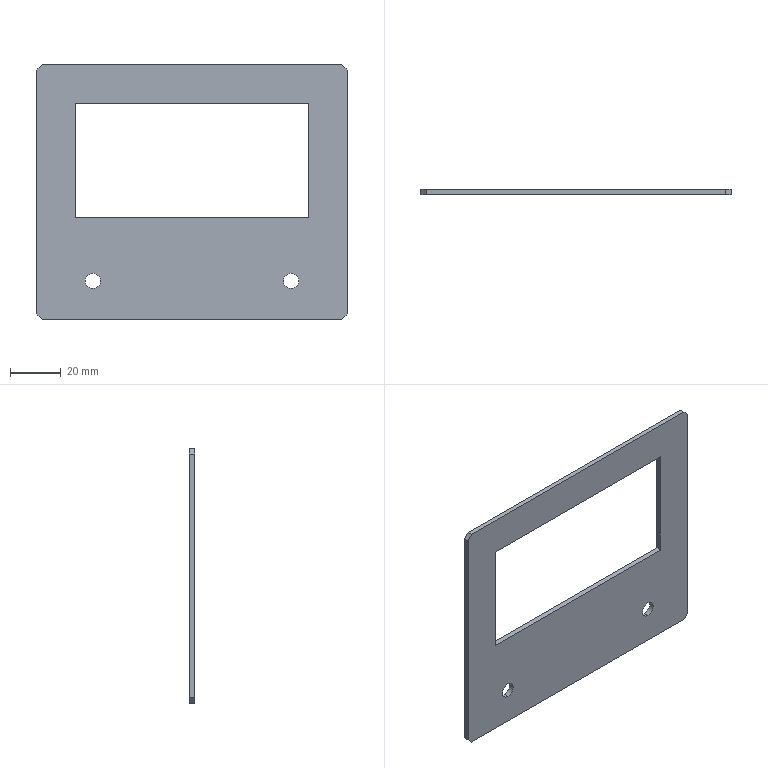Part | STEP file | 227H0563998 BKT_Default | 1 solid | 18 faces | box 122 x 2 x 100 mm | volume 15991 mm3 | plane 14 | cylinder 4 | commonest cylinder face diameters 6 x4
STEP:
#1=CARTESIAN_POINT('',(0.,0.,0.));
#2=DIRECTION('',(0.,0.,1.));
#3=DIRECTION('',(1.,0.,0.));
#4=AXIS2_PLACEMENT_3D('',#1,#2,#3);
#5=CARTESIAN_POINT('',(39.,-2.,-32.));
#6=VERTEX_POINT('',#5);
#7=CARTESIAN_POINT('',(39.,0.,-32.));
#8=VERTEX_POINT('',#7);
#9=CARTESIAN_POINT('',(39.,0.,-32.));
#10=DIRECTION('',(0.,1.,0.));
#11=VECTOR('',#10,1.);
#12=LINE('',#9,#11);
#13=CARTESIAN_POINT('',(39.,0.,-35.));
#14=DIRECTION('',(0.,1.,0.));
#15=DIRECTION('',(0.,0.,1.));
#16=AXIS2_PLACEMENT_3D('',#13,#14,#15);
#17=CYLINDRICAL_SURFACE('',#16,3.);
#18=CARTESIAN_POINT('',(6.283,0.));
#19=DIRECTION('',(0.,1.));
#20=VECTOR('',#19,1.);
#21=LINE('',#18,#20);
#22=(GEOMETRIC_REPRESENTATION_CONTEXT(2)PARAMETRIC_REPRESENTATION_CONTEXT()REPRESENTATION_CONTEXT('',''));
#23=DEFINITIONAL_REPRESENTATION('',(#21),#22);
#24=PCURVE('',#17,#23);
#25=CARTESIAN_POINT('',(39.,0.,-35.));
#26=DIRECTION('',(0.,1.,0.));
#27=DIRECTION('',(0.,0.,1.));
#28=AXIS2_PLACEMENT_3D('',#25,#26,#27);
#29=CYLINDRICAL_SURFACE('',#28,3.);
#30=CARTESIAN_POINT('',(0.,0.));
#31=DIRECTION('',(0.,1.));
#32=VECTOR('',#31,1.);
#33=LINE('',#30,#32);
#34=(GEOMETRIC_REPRESENTATION_CONTEXT(2)PARAMETRIC_REPRESENTATION_CONTEXT()REPRESENTATION_CONTEXT('',''));
#35=DEFINITIONAL_REPRESENTATION('',(#33),#34);
#36=PCURVE('',#29,#35);
#37=SURFACE_CURVE('',#12,(#24,#36),.PCURVE_S1.);
#38=EDGE_CURVE('',#6,#8,#37,.T.);
#39=ORIENTED_EDGE('',*,*,#38,.T.);
#40=CARTESIAN_POINT('',(39.,0.,-38.));
#41=VERTEX_POINT('',#40);
#42=CARTESIAN_POINT('',(39.,0.,-35.));
#43=DIRECTION('',(0.,1.,0.));
#44=DIRECTION('',(0.,0.,1.));
#45=AXIS2_PLACEMENT_3D('',#42,#43,#44);
#46=CIRCLE('',#45,3.);
#47=CARTESIAN_POINT('',(0.,0.));
#48=DIRECTION('',(1.,0.));
#49=VECTOR('',#48,1.);
#50=LINE('',#47,#49);
#51=(GEOMETRIC_REPRESENTATION_CONTEXT(2)PARAMETRIC_REPRESENTATION_CONTEXT()REPRESENTATION_CONTEXT('',''));
#52=DEFINITIONAL_REPRESENTATION('',(#50),#51);
#53=PCURVE('',#17,#52);
#54=CARTESIAN_POINT('',(0.,0.,0.));
#55=DIRECTION('',(0.,1.,0.));
#56=DIRECTION('',(0.,0.,1.));
#57=AXIS2_PLACEMENT_3D('',#54,#55,#56);
#58=PLANE('',#57);
#59=CARTESIAN_POINT('',(-35.,39.));
#60=DIRECTION('',(1.,0.));
#61=AXIS2_PLACEMENT_2D('',#59,#60);
#62=CIRCLE('',#61,3.);
#63=(GEOMETRIC_REPRESENTATION_CONTEXT(2)PARAMETRIC_REPRESENTATION_CONTEXT()REPRESENTATION_CONTEXT('',''));
#64=DEFINITIONAL_REPRESENTATION('',(#62),#63);
#65=PCURVE('',#58,#64);
#66=SURFACE_CURVE('',#46,(#53,#65),.PCURVE_S1.);
#67=EDGE_CURVE('',#41,#8,#66,.T.);
#68=ORIENTED_EDGE('',*,*,#67,.F.);
#69=CARTESIAN_POINT('',(39.,-2.,-38.));
#70=VERTEX_POINT('',#69);
#71=CARTESIAN_POINT('',(39.,0.,-38.));
#72=DIRECTION('',(0.,1.,0.));
#73=VECTOR('',#72,1.);
#74=LINE('',#71,#73);
#75=CARTESIAN_POINT('',(3.142,0.));
#76=DIRECTION('',(0.,1.));
#77=VECTOR('',#76,1.);
#78=LINE('',#75,#77);
#79=(GEOMETRIC_REPRESENTATION_CONTEXT(2)PARAMETRIC_REPRESENTATION_CONTEXT()REPRESENTATION_CONTEXT('',''));
#80=DEFINITIONAL_REPRESENTATION('',(#78),#79);
#81=PCURVE('',#17,#80);
#82=CARTESIAN_POINT('',(3.142,0.));
#83=DIRECTION('',(0.,1.));
#84=VECTOR('',#83,1.);
#85=LINE('',#82,#84);
#86=(GEOMETRIC_REPRESENTATION_CONTEXT(2)PARAMETRIC_REPRESENTATION_CONTEXT()REPRESENTATION_CONTEXT('',''));
#87=DEFINITIONAL_REPRESENTATION('',(#85),#86);
#88=PCURVE('',#29,#87);
#89=SURFACE_CURVE('',#74,(#81,#88),.PCURVE_S1.);
#90=EDGE_CURVE('',#70,#41,#89,.T.);
#91=ORIENTED_EDGE('',*,*,#90,.F.);
#92=CARTESIAN_POINT('',(39.,-2.,-35.));
#93=DIRECTION('',(0.,1.,0.));
#94=DIRECTION('',(0.,0.,1.));
#95=AXIS2_PLACEMENT_3D('',#92,#93,#94);
#96=CIRCLE('',#95,3.);
#97=CARTESIAN_POINT('',(0.,-2.));
#98=DIRECTION('',(1.,0.));
#99=VECTOR('',#98,1.);
#100=LINE('',#97,#99);
#101=(GEOMETRIC_REPRESENTATION_CONTEXT(2)PARAMETRIC_REPRESENTATION_CONTEXT()REPRESENTATION_CONTEXT('',''));
#102=DEFINITIONAL_REPRESENTATION('',(#100),#101);
#103=PCURVE('',#17,#102);
#104=CARTESIAN_POINT('',(0.,-2.,0.));
#105=DIRECTION('',(0.,1.,0.));
#106=DIRECTION('',(0.,0.,1.));
#107=AXIS2_PLACEMENT_3D('',#104,#105,#106);
#108=PLANE('',#107);
#109=CARTESIAN_POINT('',(-35.,39.));
#110=DIRECTION('',(1.,0.));
#111=AXIS2_PLACEMENT_2D('',#109,#110);
#112=CIRCLE('',#111,3.);
#113=(GEOMETRIC_REPRESENTATION_CONTEXT(2)PARAMETRIC_REPRESENTATION_CONTEXT()REPRESENTATION_CONTEXT('',''));
#114=DEFINITIONAL_REPRESENTATION('',(#112),#113);
#115=PCURVE('',#108,#114);
#116=SURFACE_CURVE('',#96,(#103,#115),.PCURVE_S1.);
#117=EDGE_CURVE('',#70,#6,#116,.T.);
#118=ORIENTED_EDGE('',*,*,#117,.T.);
#119=EDGE_LOOP('',(#39,#68,#91,#118));
#120=FACE_BOUND('',#119,.F.);
#121=ADVANCED_FACE('',(#120),#17,.F.);
#122=CARTESIAN_POINT('',(-39.,-2.,-32.));
#123=VERTEX_POINT('',#122);
#124=CARTESIAN_POINT('',(-39.,0.,-32.));
#125=VERTEX_POINT('',#124);
#126=CARTESIAN_POINT('',(-39.,0.,-32.));
#127=DIRECTION('',(0.,1.,0.));
#128=VECTOR('',#127,1.);
#129=LINE('',#126,#128);
#130=CARTESIAN_POINT('',(-39.,0.,-35.));
#131=DIRECTION('',(0.,1.,0.));
#132=DIRECTION('',(0.,0.,1.));
#133=AXIS2_PLACEMENT_3D('',#130,#131,#132);
#134=CYLINDRICAL_SURFACE('',#133,3.);
#135=CARTESIAN_POINT('',(6.283,0.));
#136=DIRECTION('',(0.,1.));
#137=VECTOR('',#136,1.);
#138=LINE('',#135,#137);
#139=(GEOMETRIC_REPRESENTATION_CONTEXT(2)PARAMETRIC_REPRESENTATION_CONTEXT()REPRESENTATION_CONTEXT('',''));
#140=DEFINITIONAL_REPRESENTATION('',(#138),#139);
#141=PCURVE('',#134,#140);
#142=CARTESIAN_POINT('',(-39.,0.,-35.));
#143=DIRECTION('',(0.,1.,0.));
#144=DIRECTION('',(0.,0.,1.));
#145=AXIS2_PLACEMENT_3D('',#142,#143,#144);
#146=CYLINDRICAL_SURFACE('',#145,3.);
#147=CARTESIAN_POINT('',(0.,0.));
#148=DIRECTION('',(0.,1.));
#149=VECTOR('',#148,1.);
#150=LINE('',#147,#149);
#151=(GEOMETRIC_REPRESENTATION_CONTEXT(2)PARAMETRIC_REPRESENTATION_CONTEXT()REPRESENTATION_CONTEXT('',''));
#152=DEFINITIONAL_REPRESENTATION('',(#150),#151);
#153=PCURVE('',#146,#152);
#154=SURFACE_CURVE('',#129,(#141,#153),.PCURVE_S1.);
#155=EDGE_CURVE('',#123,#125,#154,.T.);
#156=ORIENTED_EDGE('',*,*,#155,.T.);
#157=CARTESIAN_POINT('',(-39.,0.,-38.));
#158=VERTEX_POINT('',#157);
#159=CARTESIAN_POINT('',(-39.,0.,-35.));
#160=DIRECTION('',(0.,1.,0.));
#161=DIRECTION('',(0.,0.,1.));
#162=AXIS2_PLACEMENT_3D('',#159,#160,#161);
#163=CIRCLE('',#162,3.);
#164=CARTESIAN_POINT('',(0.,0.));
#165=DIRECTION('',(1.,0.));
#166=VECTOR('',#165,1.);
#167=LINE('',#164,#166);
#168=(GEOMETRIC_REPRESENTATION_CONTEXT(2)PARAMETRIC_REPRESENTATION_CONTEXT()REPRESENTATION_CONTEXT('',''));
#169=DEFINITIONAL_REPRESENTATION('',(#167),#168);
#170=PCURVE('',#134,#169);
#171=CARTESIAN_POINT('',(-35.,-39.));
#172=DIRECTION('',(1.,0.));
#173=AXIS2_PLACEMENT_2D('',#171,#172);
#174=CIRCLE('',#173,3.);
#175=(GEOMETRIC_REPRESENTATION_CONTEXT(2)PARAMETRIC_REPRESENTATION_CONTEXT()REPRESENTATION_CONTEXT('',''));
#176=DEFINITIONAL_REPRESENTATION('',(#174),#175);
#177=PCURVE('',#58,#176);
#178=SURFACE_CURVE('',#163,(#170,#177),.PCURVE_S1.);
#179=EDGE_CURVE('',#158,#125,#178,.T.);
#180=ORIENTED_EDGE('',*,*,#179,.F.);
#181=CARTESIAN_POINT('',(-39.,-2.,-38.));
#182=VERTEX_POINT('',#181);
#183=CARTESIAN_POINT('',(-39.,0.,-38.));
#184=DIRECTION('',(0.,1.,0.));
#185=VECTOR('',#184,1.);
#186=LINE('',#183,#185);
#187=CARTESIAN_POINT('',(3.142,0.));
#188=DIRECTION('',(0.,1.));
#189=VECTOR('',#188,1.);
#190=LINE('',#187,#189);
#191=(GEOMETRIC_REPRESENTATION_CONTEXT(2)PARAMETRIC_REPRESENTATION_CONTEXT()REPRESENTATION_CONTEXT('',''));
#192=DEFINITIONAL_REPRESENTATION('',(#190),#191);
#193=PCURVE('',#134,#192);
#194=CARTESIAN_POINT('',(3.142,0.));
#195=DIRECTION('',(0.,1.));
#196=VECTOR('',#195,1.);
#197=LINE('',#194,#196);
#198=(GEOMETRIC_REPRESENTATION_CONTEXT(2)PARAMETRIC_REPRESENTATION_CONTEXT()REPRESENTATION_CONTEXT('',''));
#199=DEFINITIONAL_REPRESENTATION('',(#197),#198);
#200=PCURVE('',#146,#199);
#201=SURFACE_CURVE('',#186,(#193,#200),.PCURVE_S1.);
#202=EDGE_CURVE('',#182,#158,#201,.T.);
#203=ORIENTED_EDGE('',*,*,#202,.F.);
#204=CARTESIAN_POINT('',(-39.,-2.,-35.));
#205=DIRECTION('',(0.,1.,0.));
#206=DIRECTION('',(0.,0.,1.));
#207=AXIS2_PLACEMENT_3D('',#204,#205,#206);
#208=CIRCLE('',#207,3.);
#209=CARTESIAN_POINT('',(0.,-2.));
#210=DIRECTION('',(1.,0.));
#211=VECTOR('',#210,1.);
#212=LINE('',#209,#211);
#213=(GEOMETRIC_REPRESENTATION_CONTEXT(2)PARAMETRIC_REPRESENTATION_CONTEXT()REPRESENTATION_CONTEXT('',''));
#214=DEFINITIONAL_REPRESENTATION('',(#212),#213);
#215=PCURVE('',#134,#214);
#216=CARTESIAN_POINT('',(-35.,-39.));
#217=DIRECTION('',(1.,0.));
#218=AXIS2_PLACEMENT_2D('',#216,#217);
#219=CIRCLE('',#218,3.);
#220=(GEOMETRIC_REPRESENTATION_CONTEXT(2)PARAMETRIC_REPRESENTATION_CONTEXT()REPRESENTATION_CONTEXT('',''));
#221=DEFINITIONAL_REPRESENTATION('',(#219),#220);
#222=PCURVE('',#108,#221);
#223=SURFACE_CURVE('',#208,(#215,#222),.PCURVE_S1.);
#224=EDGE_CURVE('',#182,#123,#223,.T.);
#225=ORIENTED_EDGE('',*,*,#224,.T.);
#226=EDGE_LOOP('',(#156,#180,#203,#225));
#227=FACE_BOUND('',#226,.F.);
#228=ADVANCED_FACE('',(#227),#134,.F.);
#229=CARTESIAN_POINT('',(-61.,0.,-48.));
#230=VERTEX_POINT('',#229);
#231=CARTESIAN_POINT('',(-61.,0.,48.));
#232=VERTEX_POINT('',#231);
#233=CARTESIAN_POINT('',(-61.,0.,50.));
#234=DIRECTION('',(0.,0.,1.));
#235=VECTOR('',#234,1.);
#236=LINE('',#233,#235);
#237=CARTESIAN_POINT('',(-61.,-2.,50.));
#238=DIRECTION('',(-1.,0.,0.));
#239=DIRECTION('',(0.,0.,1.));
#240=AXIS2_PLACEMENT_3D('',#237,#238,#239);
#241=PLANE('',#240);
#242=CARTESIAN_POINT('',(0.,2.));
#243=DIRECTION('',(1.,0.));
#244=VECTOR('',#243,1.);
#245=LINE('',#242,#244);
#246=(GEOMETRIC_REPRESENTATION_CONTEXT(2)PARAMETRIC_REPRESENTATION_CONTEXT()REPRESENTATION_CONTEXT('',''));
#247=DEFINITIONAL_REPRESENTATION('',(#245),#246);
#248=PCURVE('',#241,#247);
#249=CARTESIAN_POINT('',(50.,-61.));
#250=DIRECTION('',(1.,0.));
#251=VECTOR('',#250,1.);
#252=LINE('',#249,#251);
#253=(GEOMETRIC_REPRESENTATION_CONTEXT(2)PARAMETRIC_REPRESENTATION_CONTEXT()REPRESENTATION_CONTEXT('',''));
#254=DEFINITIONAL_REPRESENTATION('',(#252),#253);
#255=PCURVE('',#58,#254);
#256=SURFACE_CURVE('',#236,(#248,#255),.PCURVE_S1.);
#257=EDGE_CURVE('',#230,#232,#256,.T.);
#258=ORIENTED_EDGE('',*,*,#257,.F.);
#259=CARTESIAN_POINT('',(-61.,-2.,-48.));
#260=VERTEX_POINT('',#259);
#261=CARTESIAN_POINT('',(-61.,-2.,-48.));
#262=DIRECTION('',(0.,-1.,0.));
#263=VECTOR('',#262,1.);
#264=LINE('',#261,#263);
#265=CARTESIAN_POINT('',(-98.,0.));
#266=DIRECTION('',(0.,-1.));
#267=VECTOR('',#266,1.);
#268=LINE('',#265,#267);
#269=(GEOMETRIC_REPRESENTATION_CONTEXT(2)PARAMETRIC_REPRESENTATION_CONTEXT()REPRESENTATION_CONTEXT('',''));
#270=DEFINITIONAL_REPRESENTATION('',(#268),#269);
#271=PCURVE('',#241,#270);
#272=CARTESIAN_POINT('',(-59.,-2.,-50.));
#273=DIRECTION('',(0.7071,0.,0.7071));
#274=DIRECTION('',(0.,1.,0.));
#275=AXIS2_PLACEMENT_3D('',#272,#273,#274);
#276=PLANE('',#275);
#277=CARTESIAN_POINT('',(0.,2.828));
#278=DIRECTION('',(-1.,0.));
#279=VECTOR('',#278,1.);
#280=LINE('',#277,#279);
#281=(GEOMETRIC_REPRESENTATION_CONTEXT(2)PARAMETRIC_REPRESENTATION_CONTEXT()REPRESENTATION_CONTEXT('',''));
#282=DEFINITIONAL_REPRESENTATION('',(#280),#281);
#283=PCURVE('',#276,#282);
#284=SURFACE_CURVE('',#264,(#271,#283),.PCURVE_S1.);
#285=EDGE_CURVE('',#230,#260,#284,.T.);
#286=ORIENTED_EDGE('',*,*,#285,.T.);
#287=CARTESIAN_POINT('',(-61.,-2.,48.));
#288=VERTEX_POINT('',#287);
#289=CARTESIAN_POINT('',(-61.,-2.,50.));
#290=DIRECTION('',(0.,0.,1.));
#291=VECTOR('',#290,1.);
#292=LINE('',#289,#291);
#293=CARTESIAN_POINT('',(0.,0.));
#294=DIRECTION('',(1.,0.));
#295=VECTOR('',#294,1.);
#296=LINE('',#293,#295);
#297=(GEOMETRIC_REPRESENTATION_CONTEXT(2)PARAMETRIC_REPRESENTATION_CONTEXT()REPRESENTATION_CONTEXT('',''));
#298=DEFINITIONAL_REPRESENTATION('',(#296),#297);
#299=PCURVE('',#241,#298);
#300=CARTESIAN_POINT('',(50.,-61.));
#301=DIRECTION('',(1.,0.));
#302=VECTOR('',#301,1.);
#303=LINE('',#300,#302);
#304=(GEOMETRIC_REPRESENTATION_CONTEXT(2)PARAMETRIC_REPRESENTATION_CONTEXT()REPRESENTATION_CONTEXT('',''));
#305=DEFINITIONAL_REPRESENTATION('',(#303),#304);
#306=PCURVE('',#108,#305);
#307=SURFACE_CURVE('',#292,(#299,#306),.PCURVE_S1.);
#308=EDGE_CURVE('',#260,#288,#307,.T.);
#309=ORIENTED_EDGE('',*,*,#308,.T.);
#310=CARTESIAN_POINT('',(-61.,-2.,48.));
#311=DIRECTION('',(0.,1.,0.));
#312=VECTOR('',#311,1.);
#313=LINE('',#310,#312);
#314=CARTESIAN_POINT('',(-2.,0.));
#315=DIRECTION('',(0.,1.));
#316=VECTOR('',#315,1.);
#317=LINE('',#314,#316);
#318=(GEOMETRIC_REPRESENTATION_CONTEXT(2)PARAMETRIC_REPRESENTATION_CONTEXT()REPRESENTATION_CONTEXT('',''));
#319=DEFINITIONAL_REPRESENTATION('',(#317),#318);
#320=PCURVE('',#241,#319);
#321=CARTESIAN_POINT('',(-61.,-2.,48.));
#322=DIRECTION('',(0.7071,0.,-0.7071));
#323=DIRECTION('',(0.,1.,0.));
#324=AXIS2_PLACEMENT_3D('',#321,#322,#323);
#325=PLANE('',#324);
#326=CARTESIAN_POINT('',(0.,0.));
#327=DIRECTION('',(1.,0.));
#328=VECTOR('',#327,1.);
#329=LINE('',#326,#328);
#330=(GEOMETRIC_REPRESENTATION_CONTEXT(2)PARAMETRIC_REPRESENTATION_CONTEXT()REPRESENTATION_CONTEXT('',''));
#331=DEFINITIONAL_REPRESENTATION('',(#329),#330);
#332=PCURVE('',#325,#331);
#333=SURFACE_CURVE('',#313,(#320,#332),.PCURVE_S1.);
#334=EDGE_CURVE('',#288,#232,#333,.T.);
#335=ORIENTED_EDGE('',*,*,#334,.T.);
#336=EDGE_LOOP('',(#258,#286,#309,#335));
#337=FACE_BOUND('',#336,.T.);
#338=ADVANCED_FACE('',(#337),#241,.T.);
#339=CARTESIAN_POINT('',(59.,-2.,-50.));
#340=VERTEX_POINT('',#339);
#341=CARTESIAN_POINT('',(-59.,-2.,-50.));
#342=VERTEX_POINT('',#341);
#343=CARTESIAN_POINT('',(61.,-2.,-50.));
#344=DIRECTION('',(-1.,0.,0.));
#345=VECTOR('',#344,1.);
#346=LINE('',#343,#345);
#347=CARTESIAN_POINT('',(61.,-2.,-50.));
#348=DIRECTION('',(0.,0.,-1.));
#349=DIRECTION('',(-1.,0.,0.));
#350=AXIS2_PLACEMENT_3D('',#347,#348,#349);
#351=PLANE('',#350);
#352=CARTESIAN_POINT('',(0.,0.));
#353=DIRECTION('',(1.,0.));
#354=VECTOR('',#353,1.);
#355=LINE('',#352,#354);
#356=(GEOMETRIC_REPRESENTATION_CONTEXT(2)PARAMETRIC_REPRESENTATION_CONTEXT()REPRESENTATION_CONTEXT('',''));
#357=DEFINITIONAL_REPRESENTATION('',(#355),#356);
#358=PCURVE('',#351,#357);
#359=CARTESIAN_POINT('',(-50.,61.));
#360=DIRECTION('',(0.,-1.));
#361=VECTOR('',#360,1.);
#362=LINE('',#359,#361);
#363=(GEOMETRIC_REPRESENTATION_CONTEXT(2)PARAMETRIC_REPRESENTATION_CONTEXT()REPRESENTATION_CONTEXT('',''));
#364=DEFINITIONAL_REPRESENTATION('',(#362),#363);
#365=PCURVE('',#108,#364);
#366=SURFACE_CURVE('',#346,(#358,#365),.PCURVE_S1.);
#367=EDGE_CURVE('',#340,#342,#366,.T.);
#368=ORIENTED_EDGE('',*,*,#367,.T.);
#369=CARTESIAN_POINT('',(-59.,0.,-50.));
#370=VERTEX_POINT('',#369);
#371=CARTESIAN_POINT('',(-59.,-2.,-50.));
#372=DIRECTION('',(0.,1.,0.));
#373=VECTOR('',#372,1.);
#374=LINE('',#371,#373);
#375=CARTESIAN_POINT('',(120.,0.));
#376=DIRECTION('',(0.,1.));
#377=VECTOR('',#376,1.);
#378=LINE('',#375,#377);
#379=(GEOMETRIC_REPRESENTATION_CONTEXT(2)PARAMETRIC_REPRESENTATION_CONTEXT()REPRESENTATION_CONTEXT('',''));
#380=DEFINITIONAL_REPRESENTATION('',(#378),#379);
#381=PCURVE('',#351,#380);
#382=CARTESIAN_POINT('',(0.,0.));
#383=DIRECTION('',(1.,0.));
#384=VECTOR('',#383,1.);
#385=LINE('',#382,#384);
#386=(GEOMETRIC_REPRESENTATION_CONTEXT(2)PARAMETRIC_REPRESENTATION_CONTEXT()REPRESENTATION_CONTEXT('',''));
#387=DEFINITIONAL_REPRESENTATION('',(#385),#386);
#388=PCURVE('',#276,#387);
#389=SURFACE_CURVE('',#374,(#381,#388),.PCURVE_S1.);
#390=EDGE_CURVE('',#342,#370,#389,.T.);
#391=ORIENTED_EDGE('',*,*,#390,.T.);
#392=CARTESIAN_POINT('',(59.,0.,-50.));
#393=VERTEX_POINT('',#392);
#394=CARTESIAN_POINT('',(61.,0.,-50.));
#395=DIRECTION('',(-1.,0.,0.));
#396=VECTOR('',#395,1.);
#397=LINE('',#394,#396);
#398=CARTESIAN_POINT('',(0.,2.));
#399=DIRECTION('',(1.,0.));
#400=VECTOR('',#399,1.);
#401=LINE('',#398,#400);
#402=(GEOMETRIC_REPRESENTATION_CONTEXT(2)PARAMETRIC_REPRESENTATION_CONTEXT()REPRESENTATION_CONTEXT('',''));
#403=DEFINITIONAL_REPRESENTATION('',(#401),#402);
#404=PCURVE('',#351,#403);
#405=CARTESIAN_POINT('',(-50.,61.));
#406=DIRECTION('',(0.,-1.));
#407=VECTOR('',#406,1.);
#408=LINE('',#405,#407);
#409=(GEOMETRIC_REPRESENTATION_CONTEXT(2)PARAMETRIC_REPRESENTATION_CONTEXT()REPRESENTATION_CONTEXT('',''));
#410=DEFINITIONAL_REPRESENTATION('',(#408),#409);
#411=PCURVE('',#58,#410);
#412=SURFACE_CURVE('',#397,(#404,#411),.PCURVE_S1.);
#413=EDGE_CURVE('',#393,#370,#412,.T.);
#414=ORIENTED_EDGE('',*,*,#413,.F.);
#415=CARTESIAN_POINT('',(59.,-2.,-50.));
#416=DIRECTION('',(0.,-1.,0.));
#417=VECTOR('',#416,1.);
#418=LINE('',#415,#417);
#419=CARTESIAN_POINT('',(2.,0.));
#420=DIRECTION('',(0.,-1.));
#421=VECTOR('',#420,1.);
#422=LINE('',#419,#421);
#423=(GEOMETRIC_REPRESENTATION_CONTEXT(2)PARAMETRIC_REPRESENTATION_CONTEXT()REPRESENTATION_CONTEXT('',''));
#424=DEFINITIONAL_REPRESENTATION('',(#422),#423);
#425=PCURVE('',#351,#424);
#426=CARTESIAN_POINT('',(61.,-2.,-48.));
#427=DIRECTION('',(-0.7071,0.,0.7071));
#428=DIRECTION('',(0.,1.,0.));
#429=AXIS2_PLACEMENT_3D('',#426,#427,#428);
#430=PLANE('',#429);
#431=CARTESIAN_POINT('',(0.,2.828));
#432=DIRECTION('',(-1.,0.));
#433=VECTOR('',#432,1.);
#434=LINE('',#431,#433);
#435=(GEOMETRIC_REPRESENTATION_CONTEXT(2)PARAMETRIC_REPRESENTATION_CONTEXT()REPRESENTATION_CONTEXT('',''));
#436=DEFINITIONAL_REPRESENTATION('',(#434),#435);
#437=PCURVE('',#430,#436);
#438=SURFACE_CURVE('',#418,(#425,#437),.PCURVE_S1.);
#439=EDGE_CURVE('',#393,#340,#438,.T.);
#440=ORIENTED_EDGE('',*,*,#439,.T.);
#441=EDGE_LOOP('',(#368,#391,#414,#440));
#442=FACE_BOUND('',#441,.T.);
#443=ADVANCED_FACE('',(#442),#351,.T.);
#444=CARTESIAN_POINT('',(61.,-2.,48.));
#445=VERTEX_POINT('',#444);
#446=CARTESIAN_POINT('',(61.,-2.,-48.));
#447=VERTEX_POINT('',#446);
#448=CARTESIAN_POINT('',(61.,-2.,50.));
#449=DIRECTION('',(0.,0.,-1.));
#450=VECTOR('',#449,1.);
#451=LINE('',#448,#450);
#452=CARTESIAN_POINT('',(61.,-2.,50.));
#453=DIRECTION('',(1.,0.,0.));
#454=DIRECTION('',(0.,0.,-1.));
#455=AXIS2_PLACEMENT_3D('',#452,#453,#454);
#456=PLANE('',#455);
#457=CARTESIAN_POINT('',(0.,0.));
#458=DIRECTION('',(1.,0.));
#459=VECTOR('',#458,1.);
#460=LINE('',#457,#459);
#461=(GEOMETRIC_REPRESENTATION_CONTEXT(2)PARAMETRIC_REPRESENTATION_CONTEXT()REPRESENTATION_CONTEXT('',''));
#462=DEFINITIONAL_REPRESENTATION('',(#460),#461);
#463=PCURVE('',#456,#462);
#464=CARTESIAN_POINT('',(50.,61.));
#465=DIRECTION('',(-1.,0.));
#466=VECTOR('',#465,1.);
#467=LINE('',#464,#466);
#468=(GEOMETRIC_REPRESENTATION_CONTEXT(2)PARAMETRIC_REPRESENTATION_CONTEXT()REPRESENTATION_CONTEXT('',''));
#469=DEFINITIONAL_REPRESENTATION('',(#467),#468);
#470=PCURVE('',#108,#469);
#471=SURFACE_CURVE('',#451,(#463,#470),.PCURVE_S1.);
#472=EDGE_CURVE('',#445,#447,#471,.T.);
#473=ORIENTED_EDGE('',*,*,#472,.T.);
#474=CARTESIAN_POINT('',(61.,0.,-48.));
#475=VERTEX_POINT('',#474);
#476=CARTESIAN_POINT('',(61.,-2.,-48.));
#477=DIRECTION('',(0.,1.,0.));
#478=VECTOR('',#477,1.);
#479=LINE('',#476,#478);
#480=CARTESIAN_POINT('',(98.,0.));
#481=DIRECTION('',(0.,1.));
#482=VECTOR('',#481,1.);
#483=LINE('',#480,#482);
#484=(GEOMETRIC_REPRESENTATION_CONTEXT(2)PARAMETRIC_REPRESENTATION_CONTEXT()REPRESENTATION_CONTEXT('',''));
#485=DEFINITIONAL_REPRESENTATION('',(#483),#484);
#486=PCURVE('',#456,#485);
#487=CARTESIAN_POINT('',(0.,0.));
#488=DIRECTION('',(1.,0.));
#489=VECTOR('',#488,1.);
#490=LINE('',#487,#489);
#491=(GEOMETRIC_REPRESENTATION_CONTEXT(2)PARAMETRIC_REPRESENTATION_CONTEXT()REPRESENTATION_CONTEXT('',''));
#492=DEFINITIONAL_REPRESENTATION('',(#490),#491);
#493=PCURVE('',#430,#492);
#494=SURFACE_CURVE('',#479,(#486,#493),.PCURVE_S1.);
#495=EDGE_CURVE('',#447,#475,#494,.T.);
#496=ORIENTED_EDGE('',*,*,#495,.T.);
#497=CARTESIAN_POINT('',(61.,0.,48.));
#498=VERTEX_POINT('',#497);
#499=CARTESIAN_POINT('',(61.,0.,50.));
#500=DIRECTION('',(0.,0.,-1.));
#501=VECTOR('',#500,1.);
#502=LINE('',#499,#501);
#503=CARTESIAN_POINT('',(0.,2.));
#504=DIRECTION('',(1.,0.));
#505=VECTOR('',#504,1.);
#506=LINE('',#503,#505);
#507=(GEOMETRIC_REPRESENTATION_CONTEXT(2)PARAMETRIC_REPRESENTATION_CONTEXT()REPRESENTATION_CONTEXT('',''));
#508=DEFINITIONAL_REPRESENTATION('',(#506),#507);
#509=PCURVE('',#456,#508);
#510=CARTESIAN_POINT('',(50.,61.));
#511=DIRECTION('',(-1.,0.));
#512=VECTOR('',#511,1.);
#513=LINE('',#510,#512);
#514=(GEOMETRIC_REPRESENTATION_CONTEXT(2)PARAMETRIC_REPRESENTATION_CONTEXT()REPRESENTATION_CONTEXT('',''));
#515=DEFINITIONAL_REPRESENTATION('',(#513),#514);
#516=PCURVE('',#58,#515);
#517=SURFACE_CURVE('',#502,(#509,#516),.PCURVE_S1.);
#518=EDGE_CURVE('',#498,#475,#517,.T.);
#519=ORIENTED_EDGE('',*,*,#518,.F.);
#520=CARTESIAN_POINT('',(61.,-2.,48.));
#521=DIRECTION('',(0.,-1.,0.));
#522=VECTOR('',#521,1.);
#523=LINE('',#520,#522);
#524=CARTESIAN_POINT('',(2.,0.));
#525=DIRECTION('',(0.,-1.));
#526=VECTOR('',#525,1.);
#527=LINE('',#524,#526);
#528=(GEOMETRIC_REPRESENTATION_CONTEXT(2)PARAMETRIC_REPRESENTATION_CONTEXT()REPRESENTATION_CONTEXT('',''));
#529=DEFINITIONAL_REPRESENTATION('',(#527),#528);
#530=PCURVE('',#456,#529);
#531=CARTESIAN_POINT('',(59.,-2.,50.));
#532=DIRECTION('',(-0.7071,0.,-0.7071));
#533=DIRECTION('',(0.,1.,0.));
#534=AXIS2_PLACEMENT_3D('',#531,#532,#533);
#535=PLANE('',#534);
#536=CARTESIAN_POINT('',(0.,2.828));
#537=DIRECTION('',(-1.,0.));
#538=VECTOR('',#537,1.);
#539=LINE('',#536,#538);
#540=(GEOMETRIC_REPRESENTATION_CONTEXT(2)PARAMETRIC_REPRESENTATION_CONTEXT()REPRESENTATION_CONTEXT('',''));
#541=DEFINITIONAL_REPRESENTATION('',(#539),#540);
#542=PCURVE('',#535,#541);
#543=SURFACE_CURVE('',#523,(#530,#542),.PCURVE_S1.);
#544=EDGE_CURVE('',#498,#445,#543,.T.);
#545=ORIENTED_EDGE('',*,*,#544,.T.);
#546=EDGE_LOOP('',(#473,#496,#519,#545));
#547=FACE_BOUND('',#546,.T.);
#548=ADVANCED_FACE('',(#547),#456,.T.);
#549=CARTESIAN_POINT('',(-59.,-2.,50.));
#550=VERTEX_POINT('',#549);
#551=CARTESIAN_POINT('',(59.,-2.,50.));
#552=VERTEX_POINT('',#551);
#553=CARTESIAN_POINT('',(61.,-2.,50.));
#554=DIRECTION('',(1.,0.,0.));
#555=VECTOR('',#554,1.);
#556=LINE('',#553,#555);
#557=CARTESIAN_POINT('',(61.,-2.,50.));
#558=DIRECTION('',(0.,0.,1.));
#559=DIRECTION('',(1.,0.,0.));
#560=AXIS2_PLACEMENT_3D('',#557,#558,#559);
#561=PLANE('',#560);
#562=CARTESIAN_POINT('',(0.,0.));
#563=DIRECTION('',(1.,0.));
#564=VECTOR('',#563,1.);
#565=LINE('',#562,#564);
#566=(GEOMETRIC_REPRESENTATION_CONTEXT(2)PARAMETRIC_REPRESENTATION_CONTEXT()REPRESENTATION_CONTEXT('',''));
#567=DEFINITIONAL_REPRESENTATION('',(#565),#566);
#568=PCURVE('',#561,#567);
#569=CARTESIAN_POINT('',(50.,61.));
#570=DIRECTION('',(0.,1.));
#571=VECTOR('',#570,1.);
#572=LINE('',#569,#571);
#573=(GEOMETRIC_REPRESENTATION_CONTEXT(2)PARAMETRIC_REPRESENTATION_CONTEXT()REPRESENTATION_CONTEXT('',''));
#574=DEFINITIONAL_REPRESENTATION('',(#572),#573);
#575=PCURVE('',#108,#574);
#576=SURFACE_CURVE('',#556,(#568,#575),.PCURVE_S1.);
#577=EDGE_CURVE('',#550,#552,#576,.T.);
#578=ORIENTED_EDGE('',*,*,#577,.T.);
#579=CARTESIAN_POINT('',(59.,0.,50.));
#580=VERTEX_POINT('',#579);
#581=CARTESIAN_POINT('',(59.,-2.,50.));
#582=DIRECTION('',(0.,1.,0.));
#583=VECTOR('',#582,1.);
#584=LINE('',#581,#583);
#585=CARTESIAN_POINT('',(-2.,0.));
#586=DIRECTION('',(0.,1.));
#587=VECTOR('',#586,1.);
#588=LINE('',#585,#587);
#589=(GEOMETRIC_REPRESENTATION_CONTEXT(2)PARAMETRIC_REPRESENTATION_CONTEXT()REPRESENTATION_CONTEXT('',''));
#590=DEFINITIONAL_REPRESENTATION('',(#588),#589);
#591=PCURVE('',#561,#590);
#592=CARTESIAN_POINT('',(0.,0.));
#593=DIRECTION('',(1.,0.));
#594=VECTOR('',#593,1.);
#595=LINE('',#592,#594);
#596=(GEOMETRIC_REPRESENTATION_CONTEXT(2)PARAMETRIC_REPRESENTATION_CONTEXT()REPRESENTATION_CONTEXT('',''));
#597=DEFINITIONAL_REPRESENTATION('',(#595),#596);
#598=PCURVE('',#535,#597);
#599=SURFACE_CURVE('',#584,(#591,#598),.PCURVE_S1.);
#600=EDGE_CURVE('',#552,#580,#599,.T.);
#601=ORIENTED_EDGE('',*,*,#600,.T.);
#602=CARTESIAN_POINT('',(-59.,0.,50.));
#603=VERTEX_POINT('',#602);
#604=CARTESIAN_POINT('',(61.,0.,50.));
#605=DIRECTION('',(1.,0.,0.));
#606=VECTOR('',#605,1.);
#607=LINE('',#604,#606);
#608=CARTESIAN_POINT('',(0.,2.));
#609=DIRECTION('',(1.,0.));
#610=VECTOR('',#609,1.);
#611=LINE('',#608,#610);
#612=(GEOMETRIC_REPRESENTATION_CONTEXT(2)PARAMETRIC_REPRESENTATION_CONTEXT()REPRESENTATION_CONTEXT('',''));
#613=DEFINITIONAL_REPRESENTATION('',(#611),#612);
#614=PCURVE('',#561,#613);
#615=CARTESIAN_POINT('',(50.,61.));
#616=DIRECTION('',(0.,1.));
#617=VECTOR('',#616,1.);
#618=LINE('',#615,#617);
#619=(GEOMETRIC_REPRESENTATION_CONTEXT(2)PARAMETRIC_REPRESENTATION_CONTEXT()REPRESENTATION_CONTEXT('',''));
#620=DEFINITIONAL_REPRESENTATION('',(#618),#619);
#621=PCURVE('',#58,#620);
#622=SURFACE_CURVE('',#607,(#614,#621),.PCURVE_S1.);
#623=EDGE_CURVE('',#603,#580,#622,.T.);
#624=ORIENTED_EDGE('',*,*,#623,.F.);
#625=CARTESIAN_POINT('',(-59.,-2.,50.));
#626=DIRECTION('',(0.,-1.,0.));
#627=VECTOR('',#626,1.);
#628=LINE('',#625,#627);
#629=CARTESIAN_POINT('',(-120.,0.));
#630=DIRECTION('',(0.,-1.));
#631=VECTOR('',#630,1.);
#632=LINE('',#629,#631);
#633=(GEOMETRIC_REPRESENTATION_CONTEXT(2)PARAMETRIC_REPRESENTATION_CONTEXT()REPRESENTATION_CONTEXT('',''));
#634=DEFINITIONAL_REPRESENTATION('',(#632),#633);
#635=PCURVE('',#561,#634);
#636=CARTESIAN_POINT('',(0.,2.828));
#637=DIRECTION('',(-1.,0.));
#638=VECTOR('',#637,1.);
#639=LINE('',#636,#638);
#640=(GEOMETRIC_REPRESENTATION_CONTEXT(2)PARAMETRIC_REPRESENTATION_CONTEXT()REPRESENTATION_CONTEXT('',''));
#641=DEFINITIONAL_REPRESENTATION('',(#639),#640);
#642=PCURVE('',#325,#641);
#643=SURFACE_CURVE('',#628,(#635,#642),.PCURVE_S1.);
#644=EDGE_CURVE('',#603,#550,#643,.T.);
#645=ORIENTED_EDGE('',*,*,#644,.T.);
#646=EDGE_LOOP('',(#578,#601,#624,#645));
#647=FACE_BOUND('',#646,.T.);
#648=ADVANCED_FACE('',(#647),#561,.T.);
#649=CARTESIAN_POINT('',(46.,-2.,-10.));
#650=VERTEX_POINT('',#649);
#651=CARTESIAN_POINT('',(-46.,-2.,-10.));
#652=VERTEX_POINT('',#651);
#653=CARTESIAN_POINT('',(-46.,-2.,-10.));
#654=DIRECTION('',(-1.,0.,0.));
#655=VECTOR('',#654,1.);
#656=LINE('',#653,#655);
#657=CARTESIAN_POINT('',(-10.,-46.));
#658=DIRECTION('',(0.,-1.));
#659=VECTOR('',#658,1.);
#660=LINE('',#657,#659);
#661=(GEOMETRIC_REPRESENTATION_CONTEXT(2)PARAMETRIC_REPRESENTATION_CONTEXT()REPRESENTATION_CONTEXT('',''));
#662=DEFINITIONAL_REPRESENTATION('',(#660),#661);
#663=PCURVE('',#108,#662);
#664=CARTESIAN_POINT('',(-46.,-2.,-10.));
#665=DIRECTION('',(0.,0.,-1.));
#666=DIRECTION('',(-1.,0.,0.));
#667=AXIS2_PLACEMENT_3D('',#664,#665,#666);
#668=PLANE('',#667);
#669=CARTESIAN_POINT('',(0.,0.));
#670=DIRECTION('',(1.,0.));
#671=VECTOR('',#670,1.);
#672=LINE('',#669,#671);
#673=(GEOMETRIC_REPRESENTATION_CONTEXT(2)PARAMETRIC_REPRESENTATION_CONTEXT()REPRESENTATION_CONTEXT('',''));
#674=DEFINITIONAL_REPRESENTATION('',(#672),#673);
#675=PCURVE('',#668,#674);
#676=SURFACE_CURVE('',#656,(#663,#675),.PCURVE_S1.);
#677=EDGE_CURVE('',#650,#652,#676,.T.);
#678=ORIENTED_EDGE('',*,*,#677,.T.);
#679=CARTESIAN_POINT('',(-46.,-2.,35.));
#680=VERTEX_POINT('',#679);
#681=CARTESIAN_POINT('',(-46.,-2.,-10.));
#682=DIRECTION('',(0.,0.,1.));
#683=VECTOR('',#682,1.);
#684=LINE('',#681,#683);
#685=CARTESIAN_POINT('',(-10.,-46.));
#686=DIRECTION('',(1.,0.));
#687=VECTOR('',#686,1.);
#688=LINE('',#685,#687);
#689=(GEOMETRIC_REPRESENTATION_CONTEXT(2)PARAMETRIC_REPRESENTATION_CONTEXT()REPRESENTATION_CONTEXT('',''));
#690=DEFINITIONAL_REPRESENTATION('',(#688),#689);
#691=PCURVE('',#108,#690);
#692=CARTESIAN_POINT('',(-46.,-2.,-10.));
#693=DIRECTION('',(-1.,0.,0.));
#694=DIRECTION('',(0.,0.,1.));
#695=AXIS2_PLACEMENT_3D('',#692,#693,#694);
#696=PLANE('',#695);
#697=CARTESIAN_POINT('',(0.,0.));
#698=DIRECTION('',(1.,0.));
#699=VECTOR('',#698,1.);
#700=LINE('',#697,#699);
#701=(GEOMETRIC_REPRESENTATION_CONTEXT(2)PARAMETRIC_REPRESENTATION_CONTEXT()REPRESENTATION_CONTEXT('',''));
#702=DEFINITIONAL_REPRESENTATION('',(#700),#701);
#703=PCURVE('',#696,#702);
#704=SURFACE_CURVE('',#684,(#691,#703),.PCURVE_S1.);
#705=EDGE_CURVE('',#652,#680,#704,.T.);
#706=ORIENTED_EDGE('',*,*,#705,.T.);
#707=CARTESIAN_POINT('',(46.,-2.,35.));
#708=VERTEX_POINT('',#707);
#709=CARTESIAN_POINT('',(-46.,-2.,35.));
#710=DIRECTION('',(1.,0.,0.));
#711=VECTOR('',#710,1.);
#712=LINE('',#709,#711);
#713=CARTESIAN_POINT('',(35.,-46.));
#714=DIRECTION('',(0.,1.));
#715=VECTOR('',#714,1.);
#716=LINE('',#713,#715);
#717=(GEOMETRIC_REPRESENTATION_CONTEXT(2)PARAMETRIC_REPRESENTATION_CONTEXT()REPRESENTATION_CONTEXT('',''));
#718=DEFINITIONAL_REPRESENTATION('',(#716),#717);
#719=PCURVE('',#108,#718);
#720=CARTESIAN_POINT('',(-46.,-2.,35.));
#721=DIRECTION('',(0.,0.,1.));
#722=DIRECTION('',(1.,0.,0.));
#723=AXIS2_PLACEMENT_3D('',#720,#721,#722);
#724=PLANE('',#723);
#725=CARTESIAN_POINT('',(0.,0.));
#726=DIRECTION('',(1.,0.));
#727=VECTOR('',#726,1.);
#728=LINE('',#725,#727);
#729=(GEOMETRIC_REPRESENTATION_CONTEXT(2)PARAMETRIC_REPRESENTATION_CONTEXT()REPRESENTATION_CONTEXT('',''));
#730=DEFINITIONAL_REPRESENTATION('',(#728),#729);
#731=PCURVE('',#724,#730);
#732=SURFACE_CURVE('',#712,(#719,#731),.PCURVE_S1.);
#733=EDGE_CURVE('',#680,#708,#732,.T.);
#734=ORIENTED_EDGE('',*,*,#733,.T.);
#735=CARTESIAN_POINT('',(46.,-2.,-10.));
#736=DIRECTION('',(0.,0.,-1.));
#737=VECTOR('',#736,1.);
#738=LINE('',#735,#737);
#739=CARTESIAN_POINT('',(-10.,46.));
#740=DIRECTION('',(-1.,0.));
#741=VECTOR('',#740,1.);
#742=LINE('',#739,#741);
#743=(GEOMETRIC_REPRESENTATION_CONTEXT(2)PARAMETRIC_REPRESENTATION_CONTEXT()REPRESENTATION_CONTEXT('',''));
#744=DEFINITIONAL_REPRESENTATION('',(#742),#743);
#745=PCURVE('',#108,#744);
#746=CARTESIAN_POINT('',(46.,-2.,-10.));
#747=DIRECTION('',(1.,0.,0.));
#748=DIRECTION('',(0.,0.,-1.));
#749=AXIS2_PLACEMENT_3D('',#746,#747,#748);
#750=PLANE('',#749);
#751=CARTESIAN_POINT('',(0.,0.));
#752=DIRECTION('',(1.,0.));
#753=VECTOR('',#752,1.);
#754=LINE('',#751,#753);
#755=(GEOMETRIC_REPRESENTATION_CONTEXT(2)PARAMETRIC_REPRESENTATION_CONTEXT()REPRESENTATION_CONTEXT('',''));
#756=DEFINITIONAL_REPRESENTATION('',(#754),#755);
#757=PCURVE('',#750,#756);
#758=SURFACE_CURVE('',#738,(#745,#757),.PCURVE_S1.);
#759=EDGE_CURVE('',#708,#650,#758,.T.);
#760=ORIENTED_EDGE('',*,*,#759,.T.);
#761=EDGE_LOOP('',(#678,#706,#734,#760));
#762=FACE_BOUND('',#761,.T.);
#763=CARTESIAN_POINT('',(39.,-2.,-35.));
#764=DIRECTION('',(0.,1.,0.));
#765=DIRECTION('',(0.,0.,1.));
#766=AXIS2_PLACEMENT_3D('',#763,#764,#765);
#767=CIRCLE('',#766,3.);
#768=CARTESIAN_POINT('',(-35.,39.));
#769=DIRECTION('',(1.,0.));
#770=AXIS2_PLACEMENT_2D('',#768,#769);
#771=CIRCLE('',#770,3.);
#772=(GEOMETRIC_REPRESENTATION_CONTEXT(2)PARAMETRIC_REPRESENTATION_CONTEXT()REPRESENTATION_CONTEXT('',''));
#773=DEFINITIONAL_REPRESENTATION('',(#771),#772);
#774=PCURVE('',#108,#773);
#775=CARTESIAN_POINT('',(0.,-2.));
#776=DIRECTION('',(1.,0.));
#777=VECTOR('',#776,1.);
#778=LINE('',#775,#777);
#779=(GEOMETRIC_REPRESENTATION_CONTEXT(2)PARAMETRIC_REPRESENTATION_CONTEXT()REPRESENTATION_CONTEXT('',''));
#780=DEFINITIONAL_REPRESENTATION('',(#778),#779);
#781=PCURVE('',#29,#780);
#782=SURFACE_CURVE('',#767,(#774,#781),.PCURVE_S1.);
#783=EDGE_CURVE('',#6,#70,#782,.T.);
#784=ORIENTED_EDGE('',*,*,#783,.T.);
#785=ORIENTED_EDGE('',*,*,#117,.T.);
#786=EDGE_LOOP('',(#784,#785));
#787=FACE_BOUND('',#786,.T.);
#788=CARTESIAN_POINT('',(-39.,-2.,-35.));
#789=DIRECTION('',(0.,1.,0.));
#790=DIRECTION('',(0.,0.,1.));
#791=AXIS2_PLACEMENT_3D('',#788,#789,#790);
#792=CIRCLE('',#791,3.);
#793=CARTESIAN_POINT('',(-35.,-39.));
#794=DIRECTION('',(1.,0.));
#795=AXIS2_PLACEMENT_2D('',#793,#794);
#796=CIRCLE('',#795,3.);
#797=(GEOMETRIC_REPRESENTATION_CONTEXT(2)PARAMETRIC_REPRESENTATION_CONTEXT()REPRESENTATION_CONTEXT('',''));
#798=DEFINITIONAL_REPRESENTATION('',(#796),#797);
#799=PCURVE('',#108,#798);
#800=CARTESIAN_POINT('',(0.,-2.));
#801=DIRECTION('',(1.,0.));
#802=VECTOR('',#801,1.);
#803=LINE('',#800,#802);
#804=(GEOMETRIC_REPRESENTATION_CONTEXT(2)PARAMETRIC_REPRESENTATION_CONTEXT()REPRESENTATION_CONTEXT('',''));
#805=DEFINITIONAL_REPRESENTATION('',(#803),#804);
#806=PCURVE('',#146,#805);
#807=SURFACE_CURVE('',#792,(#799,#806),.PCURVE_S1.);
#808=EDGE_CURVE('',#123,#182,#807,.T.);
#809=ORIENTED_EDGE('',*,*,#808,.T.);
#810=ORIENTED_EDGE('',*,*,#224,.T.);
#811=EDGE_LOOP('',(#809,#810));
#812=FACE_BOUND('',#811,.T.);
#813=ORIENTED_EDGE('',*,*,#308,.F.);
#814=CARTESIAN_POINT('',(-59.,-2.,-50.));
#815=DIRECTION('',(0.7071,0.,-0.7071));
#816=VECTOR('',#815,1.);
#817=LINE('',#814,#816);
#818=CARTESIAN_POINT('',(-50.,-59.));
#819=DIRECTION('',(-0.7071,0.7071));
#820=VECTOR('',#819,1.);
#821=LINE('',#818,#820);
#822=(GEOMETRIC_REPRESENTATION_CONTEXT(2)PARAMETRIC_REPRESENTATION_CONTEXT()REPRESENTATION_CONTEXT('',''));
#823=DEFINITIONAL_REPRESENTATION('',(#821),#822);
#824=PCURVE('',#108,#823);
#825=CARTESIAN_POINT('',(0.,0.));
#826=DIRECTION('',(0.,-1.));
#827=VECTOR('',#826,1.);
#828=LINE('',#825,#827);
#829=(GEOMETRIC_REPRESENTATION_CONTEXT(2)PARAMETRIC_REPRESENTATION_CONTEXT()REPRESENTATION_CONTEXT('',''));
#830=DEFINITIONAL_REPRESENTATION('',(#828),#829);
#831=PCURVE('',#276,#830);
#832=SURFACE_CURVE('',#817,(#824,#831),.PCURVE_S1.);
#833=EDGE_CURVE('',#260,#342,#832,.T.);
#834=ORIENTED_EDGE('',*,*,#833,.T.);
#835=ORIENTED_EDGE('',*,*,#367,.F.);
#836=CARTESIAN_POINT('',(61.,-2.,-48.));
#837=DIRECTION('',(0.7071,0.,0.7071));
#838=VECTOR('',#837,1.);
#839=LINE('',#836,#838);
#840=CARTESIAN_POINT('',(-48.,61.));
#841=DIRECTION('',(0.7071,0.7071));
#842=VECTOR('',#841,1.);
#843=LINE('',#840,#842);
#844=(GEOMETRIC_REPRESENTATION_CONTEXT(2)PARAMETRIC_REPRESENTATION_CONTEXT()REPRESENTATION_CONTEXT('',''));
#845=DEFINITIONAL_REPRESENTATION('',(#843),#844);
#846=PCURVE('',#108,#845);
#847=CARTESIAN_POINT('',(0.,0.));
#848=DIRECTION('',(0.,-1.));
#849=VECTOR('',#848,1.);
#850=LINE('',#847,#849);
#851=(GEOMETRIC_REPRESENTATION_CONTEXT(2)PARAMETRIC_REPRESENTATION_CONTEXT()REPRESENTATION_CONTEXT('',''));
#852=DEFINITIONAL_REPRESENTATION('',(#850),#851);
#853=PCURVE('',#430,#852);
#854=SURFACE_CURVE('',#839,(#846,#853),.PCURVE_S1.);
#855=EDGE_CURVE('',#340,#447,#854,.T.);
#856=ORIENTED_EDGE('',*,*,#855,.T.);
#857=ORIENTED_EDGE('',*,*,#472,.F.);
#858=CARTESIAN_POINT('',(59.,-2.,50.));
#859=DIRECTION('',(-0.7071,0.,0.7071));
#860=VECTOR('',#859,1.);
#861=LINE('',#858,#860);
#862=CARTESIAN_POINT('',(50.,59.));
#863=DIRECTION('',(0.7071,-0.7071));
#864=VECTOR('',#863,1.);
#865=LINE('',#862,#864);
#866=(GEOMETRIC_REPRESENTATION_CONTEXT(2)PARAMETRIC_REPRESENTATION_CONTEXT()REPRESENTATION_CONTEXT('',''));
#867=DEFINITIONAL_REPRESENTATION('',(#865),#866);
#868=PCURVE('',#108,#867);
#869=CARTESIAN_POINT('',(0.,0.));
#870=DIRECTION('',(0.,-1.));
#871=VECTOR('',#870,1.);
#872=LINE('',#869,#871);
#873=(GEOMETRIC_REPRESENTATION_CONTEXT(2)PARAMETRIC_REPRESENTATION_CONTEXT()REPRESENTATION_CONTEXT('',''));
#874=DEFINITIONAL_REPRESENTATION('',(#872),#873);
#875=PCURVE('',#535,#874);
#876=SURFACE_CURVE('',#861,(#868,#875),.PCURVE_S1.);
#877=EDGE_CURVE('',#445,#552,#876,.T.);
#878=ORIENTED_EDGE('',*,*,#877,.T.);
#879=ORIENTED_EDGE('',*,*,#577,.F.);
#880=CARTESIAN_POINT('',(-61.,-2.,48.));
#881=DIRECTION('',(-0.7071,0.,-0.7071));
#882=VECTOR('',#881,1.);
#883=LINE('',#880,#882);
#884=CARTESIAN_POINT('',(48.,-61.));
#885=DIRECTION('',(-0.7071,-0.7071));
#886=VECTOR('',#885,1.);
#887=LINE('',#884,#886);
#888=(GEOMETRIC_REPRESENTATION_CONTEXT(2)PARAMETRIC_REPRESENTATION_CONTEXT()REPRESENTATION_CONTEXT('',''));
#889=DEFINITIONAL_REPRESENTATION('',(#887),#888);
#890=PCURVE('',#108,#889);
#891=CARTESIAN_POINT('',(0.,0.));
#892=DIRECTION('',(0.,-1.));
#893=VECTOR('',#892,1.);
#894=LINE('',#891,#893);
#895=(GEOMETRIC_REPRESENTATION_CONTEXT(2)PARAMETRIC_REPRESENTATION_CONTEXT()REPRESENTATION_CONTEXT('',''));
#896=DEFINITIONAL_REPRESENTATION('',(#894),#895);
#897=PCURVE('',#325,#896);
#898=SURFACE_CURVE('',#883,(#890,#897),.PCURVE_S1.);
#899=EDGE_CURVE('',#550,#288,#898,.T.);
#900=ORIENTED_EDGE('',*,*,#899,.T.);
#901=EDGE_LOOP('',(#813,#834,#835,#856,#857,#878,#879,#900));
#902=FACE_BOUND('',#901,.T.);
#903=ADVANCED_FACE('',(#762,#787,#812,#902),#108,.F.);
#904=CARTESIAN_POINT('',(-46.,0.,-10.));
#905=VERTEX_POINT('',#904);
#906=CARTESIAN_POINT('',(-46.,0.,35.));
#907=VERTEX_POINT('',#906);
#908=CARTESIAN_POINT('',(-46.,0.,-10.));
#909=DIRECTION('',(0.,0.,1.));
#910=VECTOR('',#909,1.);
#911=LINE('',#908,#910);
#912=CARTESIAN_POINT('',(-10.,-46.));
#913=DIRECTION('',(1.,0.));
#914=VECTOR('',#913,1.);
#915=LINE('',#912,#914);
#916=(GEOMETRIC_REPRESENTATION_CONTEXT(2)PARAMETRIC_REPRESENTATION_CONTEXT()REPRESENTATION_CONTEXT('',''));
#917=DEFINITIONAL_REPRESENTATION('',(#915),#916);
#918=PCURVE('',#58,#917);
#919=CARTESIAN_POINT('',(0.,2.));
#920=DIRECTION('',(1.,0.));
#921=VECTOR('',#920,1.);
#922=LINE('',#919,#921);
#923=(GEOMETRIC_REPRESENTATION_CONTEXT(2)PARAMETRIC_REPRESENTATION_CONTEXT()REPRESENTATION_CONTEXT('',''));
#924=DEFINITIONAL_REPRESENTATION('',(#922),#923);
#925=PCURVE('',#696,#924);
#926=SURFACE_CURVE('',#911,(#918,#925),.PCURVE_S1.);
#927=EDGE_CURVE('',#905,#907,#926,.T.);
#928=ORIENTED_EDGE('',*,*,#927,.F.);
#929=CARTESIAN_POINT('',(46.,0.,-10.));
#930=VERTEX_POINT('',#929);
#931=CARTESIAN_POINT('',(-46.,0.,-10.));
#932=DIRECTION('',(-1.,0.,0.));
#933=VECTOR('',#932,1.);
#934=LINE('',#931,#933);
#935=CARTESIAN_POINT('',(-10.,-46.));
#936=DIRECTION('',(0.,-1.));
#937=VECTOR('',#936,1.);
#938=LINE('',#935,#937);
#939=(GEOMETRIC_REPRESENTATION_CONTEXT(2)PARAMETRIC_REPRESENTATION_CONTEXT()REPRESENTATION_CONTEXT('',''));
#940=DEFINITIONAL_REPRESENTATION('',(#938),#939);
#941=PCURVE('',#58,#940);
#942=CARTESIAN_POINT('',(0.,2.));
#943=DIRECTION('',(1.,0.));
#944=VECTOR('',#943,1.);
#945=LINE('',#942,#944);
#946=(GEOMETRIC_REPRESENTATION_CONTEXT(2)PARAMETRIC_REPRESENTATION_CONTEXT()REPRESENTATION_CONTEXT('',''));
#947=DEFINITIONAL_REPRESENTATION('',(#945),#946);
#948=PCURVE('',#668,#947);
#949=SURFACE_CURVE('',#934,(#941,#948),.PCURVE_S1.);
#950=EDGE_CURVE('',#930,#905,#949,.T.);
#951=ORIENTED_EDGE('',*,*,#950,.F.);
#952=CARTESIAN_POINT('',(46.,0.,35.));
#953=VERTEX_POINT('',#952);
#954=CARTESIAN_POINT('',(46.,0.,-10.));
#955=DIRECTION('',(0.,0.,-1.));
#956=VECTOR('',#955,1.);
#957=LINE('',#954,#956);
#958=CARTESIAN_POINT('',(-10.,46.));
#959=DIRECTION('',(-1.,0.));
#960=VECTOR('',#959,1.);
#961=LINE('',#958,#960);
#962=(GEOMETRIC_REPRESENTATION_CONTEXT(2)PARAMETRIC_REPRESENTATION_CONTEXT()REPRESENTATION_CONTEXT('',''));
#963=DEFINITIONAL_REPRESENTATION('',(#961),#962);
#964=PCURVE('',#58,#963);
#965=CARTESIAN_POINT('',(0.,2.));
#966=DIRECTION('',(1.,0.));
#967=VECTOR('',#966,1.);
#968=LINE('',#965,#967);
#969=(GEOMETRIC_REPRESENTATION_CONTEXT(2)PARAMETRIC_REPRESENTATION_CONTEXT()REPRESENTATION_CONTEXT('',''));
#970=DEFINITIONAL_REPRESENTATION('',(#968),#969);
#971=PCURVE('',#750,#970);
#972=SURFACE_CURVE('',#957,(#964,#971),.PCURVE_S1.);
#973=EDGE_CURVE('',#953,#930,#972,.T.);
#974=ORIENTED_EDGE('',*,*,#973,.F.);
#975=CARTESIAN_POINT('',(-46.,0.,35.));
#976=DIRECTION('',(1.,0.,0.));
#977=VECTOR('',#976,1.);
#978=LINE('',#975,#977);
#979=CARTESIAN_POINT('',(35.,-46.));
#980=DIRECTION('',(0.,1.));
#981=VECTOR('',#980,1.);
#982=LINE('',#979,#981);
#983=(GEOMETRIC_REPRESENTATION_CONTEXT(2)PARAMETRIC_REPRESENTATION_CONTEXT()REPRESENTATION_CONTEXT('',''));
#984=DEFINITIONAL_REPRESENTATION('',(#982),#983);
#985=PCURVE('',#58,#984);
#986=CARTESIAN_POINT('',(0.,2.));
#987=DIRECTION('',(1.,0.));
#988=VECTOR('',#987,1.);
#989=LINE('',#986,#988);
#990=(GEOMETRIC_REPRESENTATION_CONTEXT(2)PARAMETRIC_REPRESENTATION_CONTEXT()REPRESENTATION_CONTEXT('',''));
#991=DEFINITIONAL_REPRESENTATION('',(#989),#990);
#992=PCURVE('',#724,#991);
#993=SURFACE_CURVE('',#978,(#985,#992),.PCURVE_S1.);
#994=EDGE_CURVE('',#907,#953,#993,.T.);
#995=ORIENTED_EDGE('',*,*,#994,.F.);
#996=EDGE_LOOP('',(#928,#951,#974,#995));
#997=FACE_BOUND('',#996,.T.);
#998=CARTESIAN_POINT('',(39.,0.,-35.));
#999=DIRECTION('',(0.,1.,0.));
#1000=DIRECTION('',(0.,0.,1.));
#1001=AXIS2_PLACEMENT_3D('',#998,#999,#1000);
#1002=CIRCLE('',#1001,3.);
#1003=CARTESIAN_POINT('',(-35.,39.));
#1004=DIRECTION('',(1.,0.));
#1005=AXIS2_PLACEMENT_2D('',#1003,#1004);
#1006=CIRCLE('',#1005,3.);
#1007=(GEOMETRIC_REPRESENTATION_CONTEXT(2)PARAMETRIC_REPRESENTATION_CONTEXT()REPRESENTATION_CONTEXT('',''));
#1008=DEFINITIONAL_REPRESENTATION('',(#1006),#1007);
#1009=PCURVE('',#58,#1008);
#1010=CARTESIAN_POINT('',(0.,0.));
#1011=DIRECTION('',(1.,0.));
#1012=VECTOR('',#1011,1.);
#1013=LINE('',#1010,#1012);
#1014=(GEOMETRIC_REPRESENTATION_CONTEXT(2)PARAMETRIC_REPRESENTATION_CONTEXT()REPRESENTATION_CONTEXT('',''));
#1015=DEFINITIONAL_REPRESENTATION('',(#1013),#1014);
#1016=PCURVE('',#29,#1015);
#1017=SURFACE_CURVE('',#1002,(#1009,#1016),.PCURVE_S1.);
#1018=EDGE_CURVE('',#8,#41,#1017,.T.);
#1019=ORIENTED_EDGE('',*,*,#1018,.F.);
#1020=ORIENTED_EDGE('',*,*,#67,.F.);
#1021=EDGE_LOOP('',(#1019,#1020));
#1022=FACE_BOUND('',#1021,.T.);
#1023=CARTESIAN_POINT('',(-39.,0.,-35.));
#1024=DIRECTION('',(0.,1.,0.));
#1025=DIRECTION('',(0.,0.,1.));
#1026=AXIS2_PLACEMENT_3D('',#1023,#1024,#1025);
#1027=CIRCLE('',#1026,3.);
#1028=CARTESIAN_POINT('',(-35.,-39.));
#1029=DIRECTION('',(1.,0.));
#1030=AXIS2_PLACEMENT_2D('',#1028,#1029);
#1031=CIRCLE('',#1030,3.);
#1032=(GEOMETRIC_REPRESENTATION_CONTEXT(2)PARAMETRIC_REPRESENTATION_CONTEXT()REPRESENTATION_CONTEXT('',''));
#1033=DEFINITIONAL_REPRESENTATION('',(#1031),#1032);
#1034=PCURVE('',#58,#1033);
#1035=CARTESIAN_POINT('',(0.,0.));
#1036=DIRECTION('',(1.,0.));
#1037=VECTOR('',#1036,1.);
#1038=LINE('',#1035,#1037);
#1039=(GEOMETRIC_REPRESENTATION_CONTEXT(2)PARAMETRIC_REPRESENTATION_CONTEXT()REPRESENTATION_CONTEXT('',''));
#1040=DEFINITIONAL_REPRESENTATION('',(#1038),#1039);
#1041=PCURVE('',#146,#1040);
#1042=SURFACE_CURVE('',#1027,(#1034,#1041),.PCURVE_S1.);
#1043=EDGE_CURVE('',#125,#158,#1042,.T.);
#1044=ORIENTED_EDGE('',*,*,#1043,.F.);
#1045=ORIENTED_EDGE('',*,*,#179,.F.);
#1046=EDGE_LOOP('',(#1044,#1045));
#1047=FACE_BOUND('',#1046,.T.);
#1048=ORIENTED_EDGE('',*,*,#413,.T.);
#1049=CARTESIAN_POINT('',(-54.5,0.,-54.5));
#1050=DIRECTION('',(-0.7071,0.,0.7071));
#1051=VECTOR('',#1050,1.);
#1052=LINE('',#1049,#1051);
#1053=CARTESIAN_POINT('',(-54.5,-54.5));
#1054=DIRECTION('',(0.7071,-0.7071));
#1055=VECTOR('',#1054,1.);
#1056=LINE('',#1053,#1055);
#1057=(GEOMETRIC_REPRESENTATION_CONTEXT(2)PARAMETRIC_REPRESENTATION_CONTEXT()REPRESENTATION_CONTEXT('',''));
#1058=DEFINITIONAL_REPRESENTATION('',(#1056),#1057);
#1059=PCURVE('',#58,#1058);
#1060=CARTESIAN_POINT('',(2.,-6.364));
#1061=DIRECTION('',(0.,1.));
#1062=VECTOR('',#1061,1.);
#1063=LINE('',#1060,#1062);
#1064=(GEOMETRIC_REPRESENTATION_CONTEXT(2)PARAMETRIC_REPRESENTATION_CONTEXT()REPRESENTATION_CONTEXT('',''));
#1065=DEFINITIONAL_REPRESENTATION('',(#1063),#1064);
#1066=PCURVE('',#276,#1065);
#1067=SURFACE_CURVE('',#1052,(#1059,#1066),.PCURVE_S1.);
#1068=EDGE_CURVE('',#370,#230,#1067,.T.);
#1069=ORIENTED_EDGE('',*,*,#1068,.T.);
#1070=ORIENTED_EDGE('',*,*,#257,.T.);
#1071=CARTESIAN_POINT('',(-54.5,0.,54.5));
#1072=DIRECTION('',(0.7071,0.,0.7071));
#1073=VECTOR('',#1072,1.);
#1074=LINE('',#1071,#1073);
#1075=CARTESIAN_POINT('',(54.5,-54.5));
#1076=DIRECTION('',(0.7071,0.7071));
#1077=VECTOR('',#1076,1.);
#1078=LINE('',#1075,#1077);
#1079=(GEOMETRIC_REPRESENTATION_CONTEXT(2)PARAMETRIC_REPRESENTATION_CONTEXT()REPRESENTATION_CONTEXT('',''));
#1080=DEFINITIONAL_REPRESENTATION('',(#1078),#1079);
#1081=PCURVE('',#58,#1080);
#1082=CARTESIAN_POINT('',(2.,9.192));
#1083=DIRECTION('',(0.,1.));
#1084=VECTOR('',#1083,1.);
#1085=LINE('',#1082,#1084);
#1086=(GEOMETRIC_REPRESENTATION_CONTEXT(2)PARAMETRIC_REPRESENTATION_CONTEXT()REPRESENTATION_CONTEXT('',''));
#1087=DEFINITIONAL_REPRESENTATION('',(#1085),#1086);
#1088=PCURVE('',#325,#1087);
#1089=SURFACE_CURVE('',#1074,(#1081,#1088),.PCURVE_S1.);
#1090=EDGE_CURVE('',#232,#603,#1089,.T.);
#1091=ORIENTED_EDGE('',*,*,#1090,.T.);
#1092=ORIENTED_EDGE('',*,*,#623,.T.);
#1093=CARTESIAN_POINT('',(54.5,0.,54.5));
#1094=DIRECTION('',(0.7071,0.,-0.7071));
#1095=VECTOR('',#1094,1.);
#1096=LINE('',#1093,#1095);
#1097=CARTESIAN_POINT('',(54.5,54.5));
#1098=DIRECTION('',(-0.7071,0.7071));
#1099=VECTOR('',#1098,1.);
#1100=LINE('',#1097,#1099);
#1101=(GEOMETRIC_REPRESENTATION_CONTEXT(2)PARAMETRIC_REPRESENTATION_CONTEXT()REPRESENTATION_CONTEXT('',''));
#1102=DEFINITIONAL_REPRESENTATION('',(#1100),#1101);
#1103=PCURVE('',#58,#1102);
#1104=CARTESIAN_POINT('',(2.,-6.364));
#1105=DIRECTION('',(0.,1.));
#1106=VECTOR('',#1105,1.);
#1107=LINE('',#1104,#1106);
#1108=(GEOMETRIC_REPRESENTATION_CONTEXT(2)PARAMETRIC_REPRESENTATION_CONTEXT()REPRESENTATION_CONTEXT('',''));
#1109=DEFINITIONAL_REPRESENTATION('',(#1107),#1108);
#1110=PCURVE('',#535,#1109);
#1111=SURFACE_CURVE('',#1096,(#1103,#1110),.PCURVE_S1.);
#1112=EDGE_CURVE('',#580,#498,#1111,.T.);
#1113=ORIENTED_EDGE('',*,*,#1112,.T.);
#1114=ORIENTED_EDGE('',*,*,#518,.T.);
#1115=CARTESIAN_POINT('',(54.5,0.,-54.5));
#1116=DIRECTION('',(-0.7071,0.,-0.7071));
#1117=VECTOR('',#1116,1.);
#1118=LINE('',#1115,#1117);
#1119=CARTESIAN_POINT('',(-54.5,54.5));
#1120=DIRECTION('',(-0.7071,-0.7071));
#1121=VECTOR('',#1120,1.);
#1122=LINE('',#1119,#1121);
#1123=(GEOMETRIC_REPRESENTATION_CONTEXT(2)PARAMETRIC_REPRESENTATION_CONTEXT()REPRESENTATION_CONTEXT('',''));
#1124=DEFINITIONAL_REPRESENTATION('',(#1122),#1123);
#1125=PCURVE('',#58,#1124);
#1126=CARTESIAN_POINT('',(2.,9.192));
#1127=DIRECTION('',(0.,1.));
#1128=VECTOR('',#1127,1.);
#1129=LINE('',#1126,#1128);
#1130=(GEOMETRIC_REPRESENTATION_CONTEXT(2)PARAMETRIC_REPRESENTATION_CONTEXT()REPRESENTATION_CONTEXT('',''));
#1131=DEFINITIONAL_REPRESENTATION('',(#1129),#1130);
#1132=PCURVE('',#430,#1131);
#1133=SURFACE_CURVE('',#1118,(#1125,#1132),.PCURVE_S1.);
#1134=EDGE_CURVE('',#475,#393,#1133,.T.);
#1135=ORIENTED_EDGE('',*,*,#1134,.T.);
#1136=EDGE_LOOP('',(#1048,#1069,#1070,#1091,#1092,#1113,#1114,#1135));
#1137=FACE_BOUND('',#1136,.T.);
#1138=ADVANCED_FACE('',(#997,#1022,#1047,#1137),#58,.T.);
#1139=ORIENTED_EDGE('',*,*,#1043,.F.);
#1140=ORIENTED_EDGE('',*,*,#155,.F.);
#1141=ORIENTED_EDGE('',*,*,#808,.T.);
#1142=ORIENTED_EDGE('',*,*,#202,.T.);
#1143=EDGE_LOOP('',(#1139,#1140,#1141,#1142));
#1144=FACE_BOUND('',#1143,.F.);
#1145=ADVANCED_FACE('',(#1144),#146,.F.);
#1146=ORIENTED_EDGE('',*,*,#1018,.F.);
#1147=ORIENTED_EDGE('',*,*,#38,.F.);
#1148=ORIENTED_EDGE('',*,*,#783,.T.);
#1149=ORIENTED_EDGE('',*,*,#90,.T.);
#1150=EDGE_LOOP('',(#1146,#1147,#1148,#1149));
#1151=FACE_BOUND('',#1150,.F.);
#1152=ADVANCED_FACE('',(#1151),#29,.F.);
#1153=ORIENTED_EDGE('',*,*,#927,.T.);
#1154=CARTESIAN_POINT('',(-46.,-2.,35.));
#1155=DIRECTION('',(0.,1.,0.));
#1156=VECTOR('',#1155,1.);
#1157=LINE('',#1154,#1156);
#1158=CARTESIAN_POINT('',(45.,0.));
#1159=DIRECTION('',(0.,1.));
#1160=VECTOR('',#1159,1.);
#1161=LINE('',#1158,#1160);
#1162=(GEOMETRIC_REPRESENTATION_CONTEXT(2)PARAMETRIC_REPRESENTATION_CONTEXT()REPRESENTATION_CONTEXT('',''));
#1163=DEFINITIONAL_REPRESENTATION('',(#1161),#1162);
#1164=PCURVE('',#696,#1163);
#1165=CARTESIAN_POINT('',(0.,0.));
#1166=DIRECTION('',(0.,1.));
#1167=VECTOR('',#1166,1.);
#1168=LINE('',#1165,#1167);
#1169=(GEOMETRIC_REPRESENTATION_CONTEXT(2)PARAMETRIC_REPRESENTATION_CONTEXT()REPRESENTATION_CONTEXT('',''));
#1170=DEFINITIONAL_REPRESENTATION('',(#1168),#1169);
#1171=PCURVE('',#724,#1170);
#1172=SURFACE_CURVE('',#1157,(#1164,#1171),.PCURVE_S1.);
#1173=EDGE_CURVE('',#680,#907,#1172,.T.);
#1174=ORIENTED_EDGE('',*,*,#1173,.F.);
#1175=ORIENTED_EDGE('',*,*,#705,.F.);
#1176=CARTESIAN_POINT('',(-46.,-2.,-10.));
#1177=DIRECTION('',(0.,1.,0.));
#1178=VECTOR('',#1177,1.);
#1179=LINE('',#1176,#1178);
#1180=CARTESIAN_POINT('',(0.,0.));
#1181=DIRECTION('',(0.,1.));
#1182=VECTOR('',#1181,1.);
#1183=LINE('',#1180,#1182);
#1184=(GEOMETRIC_REPRESENTATION_CONTEXT(2)PARAMETRIC_REPRESENTATION_CONTEXT()REPRESENTATION_CONTEXT('',''));
#1185=DEFINITIONAL_REPRESENTATION('',(#1183),#1184);
#1186=PCURVE('',#696,#1185);
#1187=CARTESIAN_POINT('',(0.,0.));
#1188=DIRECTION('',(0.,1.));
#1189=VECTOR('',#1188,1.);
#1190=LINE('',#1187,#1189);
#1191=(GEOMETRIC_REPRESENTATION_CONTEXT(2)PARAMETRIC_REPRESENTATION_CONTEXT()REPRESENTATION_CONTEXT('',''));
#1192=DEFINITIONAL_REPRESENTATION('',(#1190),#1191);
#1193=PCURVE('',#668,#1192);
#1194=SURFACE_CURVE('',#1179,(#1186,#1193),.PCURVE_S1.);
#1195=EDGE_CURVE('',#652,#905,#1194,.T.);
#1196=ORIENTED_EDGE('',*,*,#1195,.T.);
#1197=EDGE_LOOP('',(#1153,#1174,#1175,#1196));
#1198=FACE_BOUND('',#1197,.T.);
#1199=ADVANCED_FACE('',(#1198),#696,.F.);
#1200=ORIENTED_EDGE('',*,*,#950,.T.);
#1201=ORIENTED_EDGE('',*,*,#1195,.F.);
#1202=ORIENTED_EDGE('',*,*,#677,.F.);
#1203=CARTESIAN_POINT('',(46.,-2.,-10.));
#1204=DIRECTION('',(0.,1.,0.));
#1205=VECTOR('',#1204,1.);
#1206=LINE('',#1203,#1205);
#1207=CARTESIAN_POINT('',(-92.,0.));
#1208=DIRECTION('',(0.,1.));
#1209=VECTOR('',#1208,1.);
#1210=LINE('',#1207,#1209);
#1211=(GEOMETRIC_REPRESENTATION_CONTEXT(2)PARAMETRIC_REPRESENTATION_CONTEXT()REPRESENTATION_CONTEXT('',''));
#1212=DEFINITIONAL_REPRESENTATION('',(#1210),#1211);
#1213=PCURVE('',#668,#1212);
#1214=CARTESIAN_POINT('',(0.,0.));
#1215=DIRECTION('',(0.,1.));
#1216=VECTOR('',#1215,1.);
#1217=LINE('',#1214,#1216);
#1218=(GEOMETRIC_REPRESENTATION_CONTEXT(2)PARAMETRIC_REPRESENTATION_CONTEXT()REPRESENTATION_CONTEXT('',''));
#1219=DEFINITIONAL_REPRESENTATION('',(#1217),#1218);
#1220=PCURVE('',#750,#1219);
#1221=SURFACE_CURVE('',#1206,(#1213,#1220),.PCURVE_S1.);
#1222=EDGE_CURVE('',#650,#930,#1221,.T.);
#1223=ORIENTED_EDGE('',*,*,#1222,.T.);
#1224=EDGE_LOOP('',(#1200,#1201,#1202,#1223));
#1225=FACE_BOUND('',#1224,.T.);
#1226=ADVANCED_FACE('',(#1225),#668,.F.);
#1227=ORIENTED_EDGE('',*,*,#973,.T.);
#1228=ORIENTED_EDGE('',*,*,#1222,.F.);
#1229=ORIENTED_EDGE('',*,*,#759,.F.);
#1230=CARTESIAN_POINT('',(46.,-2.,35.));
#1231=DIRECTION('',(0.,1.,0.));
#1232=VECTOR('',#1231,1.);
#1233=LINE('',#1230,#1232);
#1234=CARTESIAN_POINT('',(-45.,0.));
#1235=DIRECTION('',(0.,1.));
#1236=VECTOR('',#1235,1.);
#1237=LINE('',#1234,#1236);
#1238=(GEOMETRIC_REPRESENTATION_CONTEXT(2)PARAMETRIC_REPRESENTATION_CONTEXT()REPRESENTATION_CONTEXT('',''));
#1239=DEFINITIONAL_REPRESENTATION('',(#1237),#1238);
#1240=PCURVE('',#750,#1239);
#1241=CARTESIAN_POINT('',(92.,0.));
#1242=DIRECTION('',(0.,1.));
#1243=VECTOR('',#1242,1.);
#1244=LINE('',#1241,#1243);
#1245=(GEOMETRIC_REPRESENTATION_CONTEXT(2)PARAMETRIC_REPRESENTATION_CONTEXT()REPRESENTATION_CONTEXT('',''));
#1246=DEFINITIONAL_REPRESENTATION('',(#1244),#1245);
#1247=PCURVE('',#724,#1246);
#1248=SURFACE_CURVE('',#1233,(#1240,#1247),.PCURVE_S1.);
#1249=EDGE_CURVE('',#708,#953,#1248,.T.);
#1250=ORIENTED_EDGE('',*,*,#1249,.T.);
#1251=EDGE_LOOP('',(#1227,#1228,#1229,#1250));
#1252=FACE_BOUND('',#1251,.T.);
#1253=ADVANCED_FACE('',(#1252),#750,.F.);
#1254=ORIENTED_EDGE('',*,*,#994,.T.);
#1255=ORIENTED_EDGE('',*,*,#1249,.F.);
#1256=ORIENTED_EDGE('',*,*,#733,.F.);
#1257=ORIENTED_EDGE('',*,*,#1173,.T.);
#1258=EDGE_LOOP('',(#1254,#1255,#1256,#1257));
#1259=FACE_BOUND('',#1258,.T.);
#1260=ADVANCED_FACE('',(#1259),#724,.F.);
#1261=ORIENTED_EDGE('',*,*,#899,.F.);
#1262=ORIENTED_EDGE('',*,*,#644,.F.);
#1263=ORIENTED_EDGE('',*,*,#1090,.F.);
#1264=ORIENTED_EDGE('',*,*,#334,.F.);
#1265=EDGE_LOOP('',(#1261,#1262,#1263,#1264));
#1266=FACE_BOUND('',#1265,.T.);
#1267=ADVANCED_FACE('',(#1266),#325,.F.);
#1268=ORIENTED_EDGE('',*,*,#877,.F.);
#1269=ORIENTED_EDGE('',*,*,#544,.F.);
#1270=ORIENTED_EDGE('',*,*,#1112,.F.);
#1271=ORIENTED_EDGE('',*,*,#600,.F.);
#1272=EDGE_LOOP('',(#1268,#1269,#1270,#1271));
#1273=FACE_BOUND('',#1272,.T.);
#1274=ADVANCED_FACE('',(#1273),#535,.F.);
#1275=ORIENTED_EDGE('',*,*,#855,.F.);
#1276=ORIENTED_EDGE('',*,*,#439,.F.);
#1277=ORIENTED_EDGE('',*,*,#1134,.F.);
#1278=ORIENTED_EDGE('',*,*,#495,.F.);
#1279=EDGE_LOOP('',(#1275,#1276,#1277,#1278));
#1280=FACE_BOUND('',#1279,.T.);
#1281=ADVANCED_FACE('',(#1280),#430,.F.);
#1282=ORIENTED_EDGE('',*,*,#833,.F.);
#1283=ORIENTED_EDGE('',*,*,#285,.F.);
#1284=ORIENTED_EDGE('',*,*,#1068,.F.);
#1285=ORIENTED_EDGE('',*,*,#390,.F.);
#1286=EDGE_LOOP('',(#1282,#1283,#1284,#1285));
#1287=FACE_BOUND('',#1286,.T.);
#1288=ADVANCED_FACE('',(#1287),#276,.F.);
#1289=CLOSED_SHELL('',(#121,#228,#338,#443,#548,#648,#903,#1138,#1145,#1152,#1199,#1226,#1253,#1260,#1267,#1274,#1281,#1288));
#1290=MANIFOLD_SOLID_BREP('',#1289);
#1291=(LENGTH_UNIT()NAMED_UNIT(*)SI_UNIT(.MILLI.,.METRE.));
#1292=UNCERTAINTY_MEASURE_WITH_UNIT(LENGTH_MEASURE(0.0000001),#1291,'','');
#1293=(NAMED_UNIT(*)PLANE_ANGLE_UNIT()SI_UNIT($,.RADIAN.));
#1294=(NAMED_UNIT(*)SI_UNIT($,.STERADIAN.)SOLID_ANGLE_UNIT());
#1295=(GEOMETRIC_REPRESENTATION_CONTEXT(3)GLOBAL_UNCERTAINTY_ASSIGNED_CONTEXT((#1292))GLOBAL_UNIT_ASSIGNED_CONTEXT((#1291,#1293,#1294))REPRESENTATION_CONTEXT('',''));
#1296=ADVANCED_BREP_SHAPE_REPRESENTATION('',(#4,#1290),#1295);